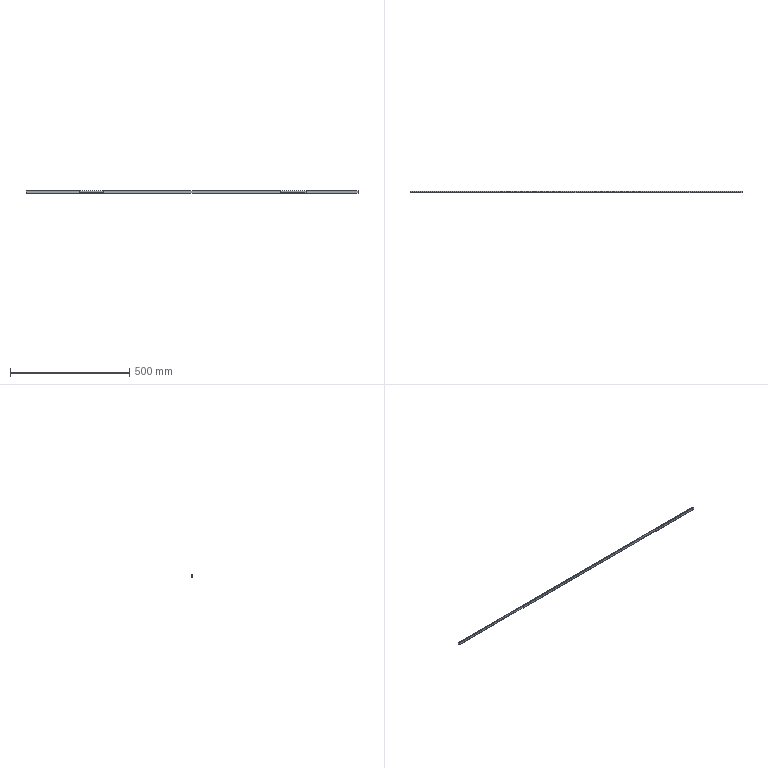Part | SolidWorks | features ICE 4, ExtruThin 1, MirrorPattern 1 | 1 solid | 23 faces | box 1390 x 5 x 10 mm | volume 29876 mm3 | plane 23
STEP:
#1=CARTESIAN_POINT('',(472.,-1.5,0.));
#2=VERTEX_POINT('',#1);
#3=CARTESIAN_POINT('',(472.,-2.5,0.));
#4=VERTEX_POINT('',#3);
#5=CARTESIAN_POINT('',(472.,-2.5,0.));
#6=DIRECTION('',(0.,-1.,0.));
#7=VECTOR('',#6,1000.);
#8=LINE('',#5,#7);
#9=EDGE_CURVE('',#2,#4,#8,.T.);
#10=ORIENTED_EDGE('',*,*,#9,.F.);
#11=CARTESIAN_POINT('',(370.,-1.5,0.));
#12=VERTEX_POINT('',#11);
#13=CARTESIAN_POINT('',(472.,-1.5,0.));
#14=DIRECTION('',(-1.,0.,0.));
#15=VECTOR('',#14,1000.);
#16=LINE('',#13,#15);
#17=EDGE_CURVE('',#2,#12,#16,.T.);
#18=ORIENTED_EDGE('',*,*,#17,.T.);
#19=CARTESIAN_POINT('',(370.,-2.5,0.));
#20=VERTEX_POINT('',#19);
#21=CARTESIAN_POINT('',(370.,-2.5,0.));
#22=DIRECTION('',(0.,-1.,0.));
#23=VECTOR('',#22,1000.);
#24=LINE('',#21,#23);
#25=EDGE_CURVE('',#12,#20,#24,.T.);
#26=ORIENTED_EDGE('',*,*,#25,.T.);
#27=CARTESIAN_POINT('',(-370.,-2.5,0.));
#28=VERTEX_POINT('',#27);
#29=CARTESIAN_POINT('',(-695.,-2.5,0.));
#30=DIRECTION('',(1.,0.,0.));
#31=VECTOR('',#30,1000.);
#32=LINE('',#29,#31);
#33=EDGE_CURVE('',#28,#20,#32,.T.);
#34=ORIENTED_EDGE('',*,*,#33,.F.);
#35=CARTESIAN_POINT('',(-370.,-1.5,0.));
#36=VERTEX_POINT('',#35);
#37=CARTESIAN_POINT('',(-370.,-2.5,0.));
#38=DIRECTION('',(0.,-1.,0.));
#39=VECTOR('',#38,1000.);
#40=LINE('',#37,#39);
#41=EDGE_CURVE('',#36,#28,#40,.T.);
#42=ORIENTED_EDGE('',*,*,#41,.F.);
#43=CARTESIAN_POINT('',(-472.,-1.5,0.));
#44=VERTEX_POINT('',#43);
#45=CARTESIAN_POINT('',(-472.,-1.5,0.));
#46=DIRECTION('',(1.,0.,0.));
#47=VECTOR('',#46,1000.);
#48=LINE('',#45,#47);
#49=EDGE_CURVE('',#44,#36,#48,.T.);
#50=ORIENTED_EDGE('',*,*,#49,.F.);
#51=CARTESIAN_POINT('',(-472.,-2.5,0.));
#52=VERTEX_POINT('',#51);
#53=CARTESIAN_POINT('',(-472.,-2.5,0.));
#54=DIRECTION('',(0.,-1.,0.));
#55=VECTOR('',#54,1000.);
#56=LINE('',#53,#55);
#57=EDGE_CURVE('',#44,#52,#56,.T.);
#58=ORIENTED_EDGE('',*,*,#57,.T.);
#59=CARTESIAN_POINT('',(-695.,-2.5,0.));
#60=VERTEX_POINT('',#59);
#61=CARTESIAN_POINT('',(-695.,-2.5,0.));
#62=DIRECTION('',(1.,0.,0.));
#63=VECTOR('',#62,1000.);
#64=LINE('',#61,#63);
#65=EDGE_CURVE('',#60,#52,#64,.T.);
#66=ORIENTED_EDGE('',*,*,#65,.F.);
#67=CARTESIAN_POINT('',(-695.,2.5,0.));
#68=VERTEX_POINT('',#67);
#69=CARTESIAN_POINT('',(-695.,-2.5,0.));
#70=DIRECTION('',(0.,-1.,0.));
#71=VECTOR('',#70,1000.);
#72=LINE('',#69,#71);
#73=EDGE_CURVE('',#68,#60,#72,.T.);
#74=ORIENTED_EDGE('',*,*,#73,.F.);
#75=CARTESIAN_POINT('',(695.,2.5,0.));
#76=VERTEX_POINT('',#75);
#77=CARTESIAN_POINT('',(-695.,2.5,0.));
#78=DIRECTION('',(-1.,0.,0.));
#79=VECTOR('',#78,1000.);
#80=LINE('',#77,#79);
#81=EDGE_CURVE('',#76,#68,#80,.T.);
#82=ORIENTED_EDGE('',*,*,#81,.F.);
#83=CARTESIAN_POINT('',(695.,-2.5,0.));
#84=VERTEX_POINT('',#83);
#85=CARTESIAN_POINT('',(695.,-2.5,0.));
#86=DIRECTION('',(0.,1.,0.));
#87=VECTOR('',#86,1000.);
#88=LINE('',#85,#87);
#89=EDGE_CURVE('',#84,#76,#88,.T.);
#90=ORIENTED_EDGE('',*,*,#89,.F.);
#91=CARTESIAN_POINT('',(-695.,-2.5,0.));
#92=DIRECTION('',(1.,0.,0.));
#93=VECTOR('',#92,1000.);
#94=LINE('',#91,#93);
#95=EDGE_CURVE('',#4,#84,#94,.T.);
#96=ORIENTED_EDGE('',*,*,#95,.F.);
#97=EDGE_LOOP('',(#10,#18,#26,#34,#42,#50,#58,#66,#74,#82,#90,#96));
#98=FACE_OUTER_BOUND('',#97,.T.);
#99=CARTESIAN_POINT('',(0.,0.,0.));
#100=DIRECTION('',(0.,0.,1.));
#101=DIRECTION('',(1.,0.,0.));
#102=AXIS2_PLACEMENT_3D('',#99,#100,#101);
#103=PLANE('',#102);
#104=ADVANCED_FACE('',(#98),#103,.F.);
#105=CARTESIAN_POINT('',(478.,-1.5,10.));
#106=VERTEX_POINT('',#105);
#107=CARTESIAN_POINT('',(478.,-2.5,10.));
#108=VERTEX_POINT('',#107);
#109=CARTESIAN_POINT('',(478.,12.317,10.));
#110=DIRECTION('',(0.,-1.,0.));
#111=VECTOR('',#110,1000.);
#112=LINE('',#109,#111);
#113=EDGE_CURVE('',#106,#108,#112,.T.);
#114=ORIENTED_EDGE('',*,*,#113,.T.);
#115=CARTESIAN_POINT('',(695.,-2.5,10.));
#116=VERTEX_POINT('',#115);
#117=CARTESIAN_POINT('',(-695.,-2.5,10.));
#118=DIRECTION('',(1.,0.,0.));
#119=VECTOR('',#118,1000.);
#120=LINE('',#117,#119);
#121=EDGE_CURVE('',#108,#116,#120,.T.);
#122=ORIENTED_EDGE('',*,*,#121,.T.);
#123=CARTESIAN_POINT('',(695.,-1.5,10.));
#124=VERTEX_POINT('',#123);
#125=CARTESIAN_POINT('',(695.,-2.5,10.));
#126=DIRECTION('',(0.,1.,0.));
#127=VECTOR('',#126,1000.);
#128=LINE('',#125,#127);
#129=EDGE_CURVE('',#116,#124,#128,.T.);
#130=ORIENTED_EDGE('',*,*,#129,.T.);
#131=CARTESIAN_POINT('',(0.,-1.5,10.));
#132=DIRECTION('',(1.,0.,0.));
#133=VECTOR('',#132,1000.);
#134=LINE('',#131,#133);
#135=EDGE_CURVE('',#106,#124,#134,.T.);
#136=ORIENTED_EDGE('',*,*,#135,.F.);
#137=EDGE_LOOP('',(#114,#122,#130,#136));
#138=FACE_OUTER_BOUND('',#137,.T.);
#139=CARTESIAN_POINT('',(0.,0.,10.));
#140=DIRECTION('',(0.,0.,1.));
#141=DIRECTION('',(1.,0.,0.));
#142=AXIS2_PLACEMENT_3D('',#139,#140,#141);
#143=PLANE('',#142);
#144=ADVANCED_FACE('',(#138),#143,.T.);
#145=CARTESIAN_POINT('',(478.,-1.5,1.));
#146=VERTEX_POINT('',#145);
#147=CARTESIAN_POINT('',(478.,-1.5,10.));
#148=DIRECTION('',(0.,0.,-1.));
#149=VECTOR('',#148,1000.);
#150=LINE('',#147,#149);
#151=EDGE_CURVE('',#106,#146,#150,.T.);
#152=ORIENTED_EDGE('',*,*,#151,.F.);
#153=ORIENTED_EDGE('',*,*,#135,.T.);
#154=CARTESIAN_POINT('',(695.,-1.5,1.));
#155=VERTEX_POINT('',#154);
#156=CARTESIAN_POINT('',(695.,-1.5,1.));
#157=DIRECTION('',(0.,0.,1.));
#158=VECTOR('',#157,1000.);
#159=LINE('',#156,#158);
#160=EDGE_CURVE('',#155,#124,#159,.T.);
#161=ORIENTED_EDGE('',*,*,#160,.F.);
#162=CARTESIAN_POINT('',(0.,-1.5,1.));
#163=DIRECTION('',(-1.,0.,0.));
#164=VECTOR('',#163,1000.);
#165=LINE('',#162,#164);
#166=EDGE_CURVE('',#155,#146,#165,.T.);
#167=ORIENTED_EDGE('',*,*,#166,.T.);
#168=EDGE_LOOP('',(#152,#153,#161,#167));
#169=FACE_OUTER_BOUND('',#168,.T.);
#170=CARTESIAN_POINT('',(0.,-1.5,10.));
#171=DIRECTION('',(0.,1.,0.));
#172=DIRECTION('',(0.,0.,1.));
#173=AXIS2_PLACEMENT_3D('',#170,#171,#172);
#174=PLANE('',#173);
#175=ADVANCED_FACE('',(#169),#174,.T.);
#176=ORIENTED_EDGE('',*,*,#121,.F.);
#177=CARTESIAN_POINT('',(478.,-2.5,1.));
#178=VERTEX_POINT('',#177);
#179=CARTESIAN_POINT('',(478.,-2.5,1.));
#180=DIRECTION('',(0.,0.,1.));
#181=VECTOR('',#180,1000.);
#182=LINE('',#179,#181);
#183=EDGE_CURVE('',#178,#108,#182,.T.);
#184=ORIENTED_EDGE('',*,*,#183,.F.);
#185=CARTESIAN_POINT('',(472.,-2.5,1.));
#186=VERTEX_POINT('',#185);
#187=CARTESIAN_POINT('',(472.,-2.5,1.));
#188=DIRECTION('',(1.,0.,0.));
#189=VECTOR('',#188,1000.);
#190=LINE('',#187,#189);
#191=EDGE_CURVE('',#186,#178,#190,.T.);
#192=ORIENTED_EDGE('',*,*,#191,.F.);
#193=CARTESIAN_POINT('',(472.,-2.5,0.));
#194=DIRECTION('',(0.,0.,1.));
#195=VECTOR('',#194,1000.);
#196=LINE('',#193,#195);
#197=EDGE_CURVE('',#4,#186,#196,.T.);
#198=ORIENTED_EDGE('',*,*,#197,.F.);
#199=ORIENTED_EDGE('',*,*,#95,.T.);
#200=CARTESIAN_POINT('',(695.,-2.5,10.));
#201=DIRECTION('',(0.,0.,-1.));
#202=VECTOR('',#201,1000.);
#203=LINE('',#200,#202);
#204=EDGE_CURVE('',#116,#84,#203,.T.);
#205=ORIENTED_EDGE('',*,*,#204,.F.);
#206=EDGE_LOOP('',(#176,#184,#192,#198,#199,#205));
#207=FACE_OUTER_BOUND('',#206,.T.);
#208=CARTESIAN_POINT('',(-695.,-2.5,10.));
#209=DIRECTION('',(0.,1.,0.));
#210=DIRECTION('',(0.,0.,1.));
#211=AXIS2_PLACEMENT_3D('',#208,#209,#210);
#212=PLANE('',#211);
#213=ADVANCED_FACE('',(#207),#212,.F.);
#214=CARTESIAN_POINT('',(-695.,-2.5,10.));
#215=VERTEX_POINT('',#214);
#216=CARTESIAN_POINT('',(-472.,-2.5,10.));
#217=VERTEX_POINT('',#216);
#218=CARTESIAN_POINT('',(-695.,-2.5,10.));
#219=DIRECTION('',(1.,0.,0.));
#220=VECTOR('',#219,1000.);
#221=LINE('',#218,#220);
#222=EDGE_CURVE('',#215,#217,#221,.T.);
#223=ORIENTED_EDGE('',*,*,#222,.T.);
#224=CARTESIAN_POINT('',(-472.,-1.5,10.));
#225=VERTEX_POINT('',#224);
#226=CARTESIAN_POINT('',(-472.,-2.5,10.));
#227=DIRECTION('',(0.,1.,0.));
#228=VECTOR('',#227,1000.);
#229=LINE('',#226,#228);
#230=EDGE_CURVE('',#217,#225,#229,.T.);
#231=ORIENTED_EDGE('',*,*,#230,.T.);
#232=CARTESIAN_POINT('',(-695.,-1.5,10.));
#233=VERTEX_POINT('',#232);
#234=CARTESIAN_POINT('',(0.,-1.5,10.));
#235=DIRECTION('',(1.,0.,0.));
#236=VECTOR('',#235,1000.);
#237=LINE('',#234,#236);
#238=EDGE_CURVE('',#233,#225,#237,.T.);
#239=ORIENTED_EDGE('',*,*,#238,.F.);
#240=CARTESIAN_POINT('',(-695.,-2.5,10.));
#241=DIRECTION('',(0.,-1.,0.));
#242=VECTOR('',#241,1000.);
#243=LINE('',#240,#242);
#244=EDGE_CURVE('',#233,#215,#243,.T.);
#245=ORIENTED_EDGE('',*,*,#244,.T.);
#246=EDGE_LOOP('',(#223,#231,#239,#245));
#247=FACE_OUTER_BOUND('',#246,.T.);
#248=CARTESIAN_POINT('',(0.,0.,10.));
#249=DIRECTION('',(0.,0.,1.));
#250=DIRECTION('',(1.,0.,0.));
#251=AXIS2_PLACEMENT_3D('',#248,#249,#250);
#252=PLANE('',#251);
#253=ADVANCED_FACE('',(#247),#252,.T.);
#254=ORIENTED_EDGE('',*,*,#238,.T.);
#255=CARTESIAN_POINT('',(-472.,-1.5,1.));
#256=VERTEX_POINT('',#255);
#257=CARTESIAN_POINT('',(-472.,-1.5,0.));
#258=DIRECTION('',(0.,0.,-1.));
#259=VECTOR('',#258,1000.);
#260=LINE('',#257,#259);
#261=EDGE_CURVE('',#225,#256,#260,.T.);
#262=ORIENTED_EDGE('',*,*,#261,.T.);
#263=CARTESIAN_POINT('',(-695.,-1.5,1.));
#264=VERTEX_POINT('',#263);
#265=CARTESIAN_POINT('',(0.,-1.5,1.));
#266=DIRECTION('',(-1.,0.,0.));
#267=VECTOR('',#266,1000.);
#268=LINE('',#265,#267);
#269=EDGE_CURVE('',#256,#264,#268,.T.);
#270=ORIENTED_EDGE('',*,*,#269,.T.);
#271=CARTESIAN_POINT('',(-695.,-1.5,1.));
#272=DIRECTION('',(0.,0.,1.));
#273=VECTOR('',#272,1000.);
#274=LINE('',#271,#273);
#275=EDGE_CURVE('',#264,#233,#274,.T.);
#276=ORIENTED_EDGE('',*,*,#275,.T.);
#277=EDGE_LOOP('',(#254,#262,#270,#276));
#278=FACE_OUTER_BOUND('',#277,.T.);
#279=CARTESIAN_POINT('',(0.,-1.5,10.));
#280=DIRECTION('',(0.,1.,0.));
#281=DIRECTION('',(0.,0.,1.));
#282=AXIS2_PLACEMENT_3D('',#279,#280,#281);
#283=PLANE('',#282);
#284=ADVANCED_FACE('',(#278),#283,.T.);
#285=CARTESIAN_POINT('',(-472.,-2.5,0.));
#286=DIRECTION('',(0.,0.,1.));
#287=VECTOR('',#286,1000.);
#288=LINE('',#285,#287);
#289=EDGE_CURVE('',#52,#217,#288,.T.);
#290=ORIENTED_EDGE('',*,*,#289,.T.);
#291=ORIENTED_EDGE('',*,*,#222,.F.);
#292=CARTESIAN_POINT('',(-695.,-2.5,10.));
#293=DIRECTION('',(0.,0.,-1.));
#294=VECTOR('',#293,1000.);
#295=LINE('',#292,#294);
#296=EDGE_CURVE('',#215,#60,#295,.T.);
#297=ORIENTED_EDGE('',*,*,#296,.T.);
#298=ORIENTED_EDGE('',*,*,#65,.T.);
#299=EDGE_LOOP('',(#290,#291,#297,#298));
#300=FACE_OUTER_BOUND('',#299,.T.);
#301=CARTESIAN_POINT('',(-695.,-2.5,10.));
#302=DIRECTION('',(0.,1.,0.));
#303=DIRECTION('',(0.,0.,1.));
#304=AXIS2_PLACEMENT_3D('',#301,#302,#303);
#305=PLANE('',#304);
#306=ADVANCED_FACE('',(#300),#305,.F.);
#307=CARTESIAN_POINT('',(370.,-2.5,10.));
#308=VERTEX_POINT('',#307);
#309=CARTESIAN_POINT('',(370.,-1.5,10.));
#310=VERTEX_POINT('',#309);
#311=CARTESIAN_POINT('',(370.,-2.5,10.));
#312=DIRECTION('',(0.,1.,0.));
#313=VECTOR('',#312,1000.);
#314=LINE('',#311,#313);
#315=EDGE_CURVE('',#308,#310,#314,.T.);
#316=ORIENTED_EDGE('',*,*,#315,.T.);
#317=CARTESIAN_POINT('',(-370.,-1.5,10.));
#318=VERTEX_POINT('',#317);
#319=CARTESIAN_POINT('',(0.,-1.5,10.));
#320=DIRECTION('',(1.,0.,0.));
#321=VECTOR('',#320,1000.);
#322=LINE('',#319,#321);
#323=EDGE_CURVE('',#318,#310,#322,.T.);
#324=ORIENTED_EDGE('',*,*,#323,.F.);
#325=CARTESIAN_POINT('',(-370.,-2.5,10.));
#326=VERTEX_POINT('',#325);
#327=CARTESIAN_POINT('',(-370.,-2.5,10.));
#328=DIRECTION('',(0.,1.,0.));
#329=VECTOR('',#328,1000.);
#330=LINE('',#327,#329);
#331=EDGE_CURVE('',#326,#318,#330,.T.);
#332=ORIENTED_EDGE('',*,*,#331,.F.);
#333=CARTESIAN_POINT('',(-695.,-2.5,10.));
#334=DIRECTION('',(1.,0.,0.));
#335=VECTOR('',#334,1000.);
#336=LINE('',#333,#335);
#337=EDGE_CURVE('',#326,#308,#336,.T.);
#338=ORIENTED_EDGE('',*,*,#337,.T.);
#339=EDGE_LOOP('',(#316,#324,#332,#338));
#340=FACE_OUTER_BOUND('',#339,.T.);
#341=CARTESIAN_POINT('',(0.,0.,10.));
#342=DIRECTION('',(0.,0.,1.));
#343=DIRECTION('',(1.,0.,0.));
#344=AXIS2_PLACEMENT_3D('',#341,#342,#343);
#345=PLANE('',#344);
#346=ADVANCED_FACE('',(#340),#345,.T.);
#347=CARTESIAN_POINT('',(695.,1.5,10.));
#348=VERTEX_POINT('',#347);
#349=CARTESIAN_POINT('',(-695.,1.5,10.));
#350=VERTEX_POINT('',#349);
#351=CARTESIAN_POINT('',(0.,1.5,10.));
#352=DIRECTION('',(-1.,0.,0.));
#353=VECTOR('',#352,1000.);
#354=LINE('',#351,#353);
#355=EDGE_CURVE('',#348,#350,#354,.T.);
#356=ORIENTED_EDGE('',*,*,#355,.T.);
#357=CARTESIAN_POINT('',(-695.,1.5,1.));
#358=VERTEX_POINT('',#357);
#359=CARTESIAN_POINT('',(-695.,1.5,10.));
#360=DIRECTION('',(0.,0.,-1.));
#361=VECTOR('',#360,1000.);
#362=LINE('',#359,#361);
#363=EDGE_CURVE('',#350,#358,#362,.T.);
#364=ORIENTED_EDGE('',*,*,#363,.T.);
#365=CARTESIAN_POINT('',(695.,1.5,1.));
#366=VERTEX_POINT('',#365);
#367=CARTESIAN_POINT('',(0.,1.5,1.));
#368=DIRECTION('',(1.,0.,0.));
#369=VECTOR('',#368,1000.);
#370=LINE('',#367,#369);
#371=EDGE_CURVE('',#358,#366,#370,.T.);
#372=ORIENTED_EDGE('',*,*,#371,.T.);
#373=CARTESIAN_POINT('',(695.,1.5,10.));
#374=DIRECTION('',(0.,0.,-1.));
#375=VECTOR('',#374,1000.);
#376=LINE('',#373,#375);
#377=EDGE_CURVE('',#348,#366,#376,.T.);
#378=ORIENTED_EDGE('',*,*,#377,.F.);
#379=EDGE_LOOP('',(#356,#364,#372,#378));
#380=FACE_OUTER_BOUND('',#379,.T.);
#381=CARTESIAN_POINT('',(0.,1.5,10.));
#382=DIRECTION('',(0.,-1.,0.));
#383=DIRECTION('',(0.,0.,-1.));
#384=AXIS2_PLACEMENT_3D('',#381,#382,#383);
#385=PLANE('',#384);
#386=ADVANCED_FACE('',(#380),#385,.T.);
#387=CARTESIAN_POINT('',(370.,-1.5,1.));
#388=VERTEX_POINT('',#387);
#389=CARTESIAN_POINT('',(370.,-1.5,0.));
#390=DIRECTION('',(0.,0.,-1.));
#391=VECTOR('',#390,1000.);
#392=LINE('',#389,#391);
#393=EDGE_CURVE('',#310,#388,#392,.T.);
#394=ORIENTED_EDGE('',*,*,#393,.T.);
#395=CARTESIAN_POINT('',(-370.,-1.5,1.));
#396=VERTEX_POINT('',#395);
#397=CARTESIAN_POINT('',(0.,-1.5,1.));
#398=DIRECTION('',(-1.,0.,0.));
#399=VECTOR('',#398,1000.);
#400=LINE('',#397,#399);
#401=EDGE_CURVE('',#388,#396,#400,.T.);
#402=ORIENTED_EDGE('',*,*,#401,.T.);
#403=CARTESIAN_POINT('',(-370.,-1.5,0.));
#404=DIRECTION('',(0.,0.,-1.));
#405=VECTOR('',#404,1000.);
#406=LINE('',#403,#405);
#407=EDGE_CURVE('',#318,#396,#406,.T.);
#408=ORIENTED_EDGE('',*,*,#407,.F.);
#409=ORIENTED_EDGE('',*,*,#323,.T.);
#410=EDGE_LOOP('',(#394,#402,#408,#409));
#411=FACE_OUTER_BOUND('',#410,.T.);
#412=CARTESIAN_POINT('',(0.,-1.5,10.));
#413=DIRECTION('',(0.,1.,0.));
#414=DIRECTION('',(0.,0.,1.));
#415=AXIS2_PLACEMENT_3D('',#412,#413,#414);
#416=PLANE('',#415);
#417=ADVANCED_FACE('',(#411),#416,.T.);
#418=ORIENTED_EDGE('',*,*,#355,.F.);
#419=CARTESIAN_POINT('',(695.,2.5,10.));
#420=VERTEX_POINT('',#419);
#421=CARTESIAN_POINT('',(695.,-2.5,10.));
#422=DIRECTION('',(0.,1.,0.));
#423=VECTOR('',#422,1000.);
#424=LINE('',#421,#423);
#425=EDGE_CURVE('',#348,#420,#424,.T.);
#426=ORIENTED_EDGE('',*,*,#425,.T.);
#427=CARTESIAN_POINT('',(-695.,2.5,10.));
#428=VERTEX_POINT('',#427);
#429=CARTESIAN_POINT('',(-695.,2.5,10.));
#430=DIRECTION('',(-1.,0.,0.));
#431=VECTOR('',#430,1000.);
#432=LINE('',#429,#431);
#433=EDGE_CURVE('',#420,#428,#432,.T.);
#434=ORIENTED_EDGE('',*,*,#433,.T.);
#435=CARTESIAN_POINT('',(-695.,-2.5,10.));
#436=DIRECTION('',(0.,-1.,0.));
#437=VECTOR('',#436,1000.);
#438=LINE('',#435,#437);
#439=EDGE_CURVE('',#428,#350,#438,.T.);
#440=ORIENTED_EDGE('',*,*,#439,.T.);
#441=EDGE_LOOP('',(#418,#426,#434,#440));
#442=FACE_OUTER_BOUND('',#441,.T.);
#443=CARTESIAN_POINT('',(0.,0.,10.));
#444=DIRECTION('',(0.,0.,1.));
#445=DIRECTION('',(1.,0.,0.));
#446=AXIS2_PLACEMENT_3D('',#443,#444,#445);
#447=PLANE('',#446);
#448=ADVANCED_FACE('',(#442),#447,.T.);
#449=CARTESIAN_POINT('',(695.,1.5,1.));
#450=DIRECTION('',(0.,-1.,0.));
#451=VECTOR('',#450,1000.);
#452=LINE('',#449,#451);
#453=EDGE_CURVE('',#366,#155,#452,.T.);
#454=ORIENTED_EDGE('',*,*,#453,.T.);
#455=ORIENTED_EDGE('',*,*,#160,.T.);
#456=ORIENTED_EDGE('',*,*,#129,.F.);
#457=ORIENTED_EDGE('',*,*,#204,.T.);
#458=ORIENTED_EDGE('',*,*,#89,.T.);
#459=CARTESIAN_POINT('',(695.,2.5,10.));
#460=DIRECTION('',(0.,0.,-1.));
#461=VECTOR('',#460,1000.);
#462=LINE('',#459,#461);
#463=EDGE_CURVE('',#420,#76,#462,.T.);
#464=ORIENTED_EDGE('',*,*,#463,.F.);
#465=ORIENTED_EDGE('',*,*,#425,.F.);
#466=ORIENTED_EDGE('',*,*,#377,.T.);
#467=EDGE_LOOP('',(#454,#455,#456,#457,#458,#464,#465,#466));
#468=FACE_OUTER_BOUND('',#467,.T.);
#469=CARTESIAN_POINT('',(695.,-2.5,10.));
#470=DIRECTION('',(-1.,0.,0.));
#471=DIRECTION('',(0.,0.,1.));
#472=AXIS2_PLACEMENT_3D('',#469,#470,#471);
#473=PLANE('',#472);
#474=ADVANCED_FACE('',(#468),#473,.F.);
#475=ORIENTED_EDGE('',*,*,#81,.T.);
#476=CARTESIAN_POINT('',(-695.,2.5,10.));
#477=DIRECTION('',(0.,0.,-1.));
#478=VECTOR('',#477,1000.);
#479=LINE('',#476,#478);
#480=EDGE_CURVE('',#428,#68,#479,.T.);
#481=ORIENTED_EDGE('',*,*,#480,.F.);
#482=ORIENTED_EDGE('',*,*,#433,.F.);
#483=ORIENTED_EDGE('',*,*,#463,.T.);
#484=EDGE_LOOP('',(#475,#481,#482,#483));
#485=FACE_OUTER_BOUND('',#484,.T.);
#486=CARTESIAN_POINT('',(-695.,2.5,10.));
#487=DIRECTION('',(0.,-1.,0.));
#488=DIRECTION('',(0.,0.,-1.));
#489=AXIS2_PLACEMENT_3D('',#486,#487,#488);
#490=PLANE('',#489);
#491=ADVANCED_FACE('',(#485),#490,.F.);
#492=ORIENTED_EDGE('',*,*,#244,.F.);
#493=ORIENTED_EDGE('',*,*,#275,.F.);
#494=CARTESIAN_POINT('',(-695.,1.5,1.));
#495=DIRECTION('',(0.,-1.,0.));
#496=VECTOR('',#495,1000.);
#497=LINE('',#494,#496);
#498=EDGE_CURVE('',#358,#264,#497,.T.);
#499=ORIENTED_EDGE('',*,*,#498,.F.);
#500=ORIENTED_EDGE('',*,*,#363,.F.);
#501=ORIENTED_EDGE('',*,*,#439,.F.);
#502=ORIENTED_EDGE('',*,*,#480,.T.);
#503=ORIENTED_EDGE('',*,*,#73,.T.);
#504=ORIENTED_EDGE('',*,*,#296,.F.);
#505=EDGE_LOOP('',(#492,#493,#499,#500,#501,#502,#503,#504));
#506=FACE_OUTER_BOUND('',#505,.T.);
#507=CARTESIAN_POINT('',(-695.,-2.5,10.));
#508=DIRECTION('',(1.,0.,0.));
#509=DIRECTION('',(0.,0.,-1.));
#510=AXIS2_PLACEMENT_3D('',#507,#508,#509);
#511=PLANE('',#510);
#512=ADVANCED_FACE('',(#506),#511,.F.);
#513=ORIENTED_EDGE('',*,*,#33,.T.);
#514=CARTESIAN_POINT('',(370.,-2.5,0.));
#515=DIRECTION('',(0.,0.,1.));
#516=VECTOR('',#515,1000.);
#517=LINE('',#514,#516);
#518=EDGE_CURVE('',#20,#308,#517,.T.);
#519=ORIENTED_EDGE('',*,*,#518,.T.);
#520=ORIENTED_EDGE('',*,*,#337,.F.);
#521=CARTESIAN_POINT('',(-370.,-2.5,0.));
#522=DIRECTION('',(0.,0.,1.));
#523=VECTOR('',#522,1000.);
#524=LINE('',#521,#523);
#525=EDGE_CURVE('',#28,#326,#524,.T.);
#526=ORIENTED_EDGE('',*,*,#525,.F.);
#527=EDGE_LOOP('',(#513,#519,#520,#526));
#528=FACE_OUTER_BOUND('',#527,.T.);
#529=CARTESIAN_POINT('',(-695.,-2.5,10.));
#530=DIRECTION('',(0.,1.,0.));
#531=DIRECTION('',(0.,0.,1.));
#532=AXIS2_PLACEMENT_3D('',#529,#530,#531);
#533=PLANE('',#532);
#534=ADVANCED_FACE('',(#528),#533,.F.);
#535=ORIENTED_EDGE('',*,*,#453,.F.);
#536=ORIENTED_EDGE('',*,*,#371,.F.);
#537=ORIENTED_EDGE('',*,*,#498,.T.);
#538=ORIENTED_EDGE('',*,*,#269,.F.);
#539=CARTESIAN_POINT('',(0.,-1.5,1.));
#540=DIRECTION('',(-1.,0.,0.));
#541=VECTOR('',#540,1000.);
#542=LINE('',#539,#541);
#543=EDGE_CURVE('',#396,#256,#542,.T.);
#544=ORIENTED_EDGE('',*,*,#543,.F.);
#545=ORIENTED_EDGE('',*,*,#401,.F.);
#546=CARTESIAN_POINT('',(472.,-1.5,1.));
#547=VERTEX_POINT('',#546);
#548=CARTESIAN_POINT('',(0.,-1.5,1.));
#549=DIRECTION('',(-1.,0.,0.));
#550=VECTOR('',#549,1000.);
#551=LINE('',#548,#550);
#552=EDGE_CURVE('',#547,#388,#551,.T.);
#553=ORIENTED_EDGE('',*,*,#552,.F.);
#554=CARTESIAN_POINT('',(472.,0.,1.));
#555=DIRECTION('',(0.,-1.,0.));
#556=VECTOR('',#555,1000.);
#557=LINE('',#554,#556);
#558=EDGE_CURVE('',#547,#186,#557,.T.);
#559=ORIENTED_EDGE('',*,*,#558,.T.);
#560=ORIENTED_EDGE('',*,*,#191,.T.);
#561=CARTESIAN_POINT('',(478.,12.317,1.));
#562=DIRECTION('',(0.,-1.,0.));
#563=VECTOR('',#562,1000.);
#564=LINE('',#561,#563);
#565=EDGE_CURVE('',#146,#178,#564,.T.);
#566=ORIENTED_EDGE('',*,*,#565,.F.);
#567=ORIENTED_EDGE('',*,*,#166,.F.);
#568=EDGE_LOOP('',(#535,#536,#537,#538,#544,#545,#553,#559,#560,#566,#567));
#569=FACE_OUTER_BOUND('',#568,.T.);
#570=CARTESIAN_POINT('',(699.099,2.5,1.));
#571=DIRECTION('',(0.,0.,-1.));
#572=DIRECTION('',(0.,1.,0.));
#573=AXIS2_PLACEMENT_3D('',#570,#571,#572);
#574=PLANE('',#573);
#575=ADVANCED_FACE('',(#569),#574,.F.);
#576=ORIENTED_EDGE('',*,*,#543,.T.);
#577=CARTESIAN_POINT('',(-472.,-1.5,0.));
#578=DIRECTION('',(0.,0.,-1.));
#579=VECTOR('',#578,1000.);
#580=LINE('',#577,#579);
#581=EDGE_CURVE('',#256,#44,#580,.T.);
#582=ORIENTED_EDGE('',*,*,#581,.T.);
#583=ORIENTED_EDGE('',*,*,#49,.T.);
#584=CARTESIAN_POINT('',(-370.,-1.5,0.));
#585=DIRECTION('',(0.,0.,-1.));
#586=VECTOR('',#585,1000.);
#587=LINE('',#584,#586);
#588=EDGE_CURVE('',#396,#36,#587,.T.);
#589=ORIENTED_EDGE('',*,*,#588,.F.);
#590=EDGE_LOOP('',(#576,#582,#583,#589));
#591=FACE_OUTER_BOUND('',#590,.T.);
#592=CARTESIAN_POINT('',(-472.,-1.5,0.));
#593=DIRECTION('',(0.,-1.,0.));
#594=DIRECTION('',(0.,0.,-1.));
#595=AXIS2_PLACEMENT_3D('',#592,#593,#594);
#596=PLANE('',#595);
#597=ADVANCED_FACE('',(#591),#596,.T.);
#598=ORIENTED_EDGE('',*,*,#57,.F.);
#599=ORIENTED_EDGE('',*,*,#581,.F.);
#600=ORIENTED_EDGE('',*,*,#261,.F.);
#601=ORIENTED_EDGE('',*,*,#230,.F.);
#602=ORIENTED_EDGE('',*,*,#289,.F.);
#603=EDGE_LOOP('',(#598,#599,#600,#601,#602));
#604=FACE_OUTER_BOUND('',#603,.T.);
#605=CARTESIAN_POINT('',(-472.,0.,0.));
#606=DIRECTION('',(1.,0.,0.));
#607=DIRECTION('',(0.,0.,-1.));
#608=AXIS2_PLACEMENT_3D('',#605,#606,#607);
#609=PLANE('',#608);
#610=ADVANCED_FACE('',(#604),#609,.T.);
#611=ORIENTED_EDGE('',*,*,#41,.T.);
#612=ORIENTED_EDGE('',*,*,#525,.T.);
#613=ORIENTED_EDGE('',*,*,#331,.T.);
#614=ORIENTED_EDGE('',*,*,#407,.T.);
#615=ORIENTED_EDGE('',*,*,#588,.T.);
#616=EDGE_LOOP('',(#611,#612,#613,#614,#615));
#617=FACE_OUTER_BOUND('',#616,.T.);
#618=CARTESIAN_POINT('',(-370.,0.,0.));
#619=DIRECTION('',(1.,0.,0.));
#620=DIRECTION('',(0.,0.,-1.));
#621=AXIS2_PLACEMENT_3D('',#618,#619,#620);
#622=PLANE('',#621);
#623=ADVANCED_FACE('',(#617),#622,.F.);
#624=CARTESIAN_POINT('',(370.,-1.5,0.));
#625=DIRECTION('',(0.,0.,-1.));
#626=VECTOR('',#625,1000.);
#627=LINE('',#624,#626);
#628=EDGE_CURVE('',#388,#12,#627,.T.);
#629=ORIENTED_EDGE('',*,*,#628,.T.);
#630=ORIENTED_EDGE('',*,*,#17,.F.);
#631=CARTESIAN_POINT('',(472.,-1.5,0.));
#632=DIRECTION('',(0.,0.,-1.));
#633=VECTOR('',#632,1000.);
#634=LINE('',#631,#633);
#635=EDGE_CURVE('',#547,#2,#634,.T.);
#636=ORIENTED_EDGE('',*,*,#635,.F.);
#637=ORIENTED_EDGE('',*,*,#552,.T.);
#638=EDGE_LOOP('',(#629,#630,#636,#637));
#639=FACE_OUTER_BOUND('',#638,.T.);
#640=CARTESIAN_POINT('',(472.,-1.5,0.));
#641=DIRECTION('',(0.,1.,0.));
#642=DIRECTION('',(0.,0.,1.));
#643=AXIS2_PLACEMENT_3D('',#640,#641,#642);
#644=PLANE('',#643);
#645=ADVANCED_FACE('',(#639),#644,.F.);
#646=ORIENTED_EDGE('',*,*,#558,.F.);
#647=ORIENTED_EDGE('',*,*,#635,.T.);
#648=ORIENTED_EDGE('',*,*,#9,.T.);
#649=ORIENTED_EDGE('',*,*,#197,.T.);
#650=EDGE_LOOP('',(#646,#647,#648,#649));
#651=FACE_OUTER_BOUND('',#650,.T.);
#652=CARTESIAN_POINT('',(472.,0.,0.));
#653=DIRECTION('',(-1.,0.,0.));
#654=DIRECTION('',(0.,0.,-1.));
#655=AXIS2_PLACEMENT_3D('',#652,#653,#654);
#656=PLANE('',#655);
#657=ADVANCED_FACE('',(#651),#656,.T.);
#658=ORIENTED_EDGE('',*,*,#25,.F.);
#659=ORIENTED_EDGE('',*,*,#628,.F.);
#660=ORIENTED_EDGE('',*,*,#393,.F.);
#661=ORIENTED_EDGE('',*,*,#315,.F.);
#662=ORIENTED_EDGE('',*,*,#518,.F.);
#663=EDGE_LOOP('',(#658,#659,#660,#661,#662));
#664=FACE_OUTER_BOUND('',#663,.T.);
#665=CARTESIAN_POINT('',(370.,0.,0.));
#666=DIRECTION('',(-1.,0.,0.));
#667=DIRECTION('',(0.,0.,-1.));
#668=AXIS2_PLACEMENT_3D('',#665,#666,#667);
#669=PLANE('',#668);
#670=ADVANCED_FACE('',(#664),#669,.F.);
#671=ORIENTED_EDGE('',*,*,#151,.T.);
#672=ORIENTED_EDGE('',*,*,#565,.T.);
#673=ORIENTED_EDGE('',*,*,#183,.T.);
#674=ORIENTED_EDGE('',*,*,#113,.F.);
#675=EDGE_LOOP('',(#671,#672,#673,#674));
#676=FACE_OUTER_BOUND('',#675,.T.);
#677=CARTESIAN_POINT('',(478.,12.317,1.));
#678=DIRECTION('',(1.,0.,0.));
#679=DIRECTION('',(0.,0.,-1.));
#680=AXIS2_PLACEMENT_3D('',#677,#678,#679);
#681=PLANE('',#680);
#682=ADVANCED_FACE('',(#676),#681,.F.);
#683=CLOSED_SHELL('',(#104,#144,#175,#213,#253,#284,#306,#346,#386,#417,#448,#474,#491,#512,#534,#575,#597,#610,#623,#645,#657,#670,#682));
#684=MANIFOLD_SOLID_BREP('',#683);
#685=CARTESIAN_POINT('',(0.,0.,0.));
#686=DIRECTION('',(0.,0.,1.));
#687=DIRECTION('',(1.,0.,0.));
#688=AXIS2_PLACEMENT_3D('',#685,#686,#687);
#689=(LENGTH_UNIT()NAMED_UNIT(*)SI_UNIT(.MILLI.,.METRE.));
#690=UNCERTAINTY_MEASURE_WITH_UNIT(LENGTH_MEASURE(0.00001),#689,'','');
#691=(NAMED_UNIT(*)PLANE_ANGLE_UNIT()SI_UNIT($,.RADIAN.));
#692=(NAMED_UNIT(*)SI_UNIT($,.STERADIAN.)SOLID_ANGLE_UNIT());
#693=(GEOMETRIC_REPRESENTATION_CONTEXT(3)GLOBAL_UNCERTAINTY_ASSIGNED_CONTEXT((#690))GLOBAL_UNIT_ASSIGNED_CONTEXT((#689,#691,#692))REPRESENTATION_CONTEXT('',''));
#694=ADVANCED_BREP_SHAPE_REPRESENTATION('',(#684,#688),#693);